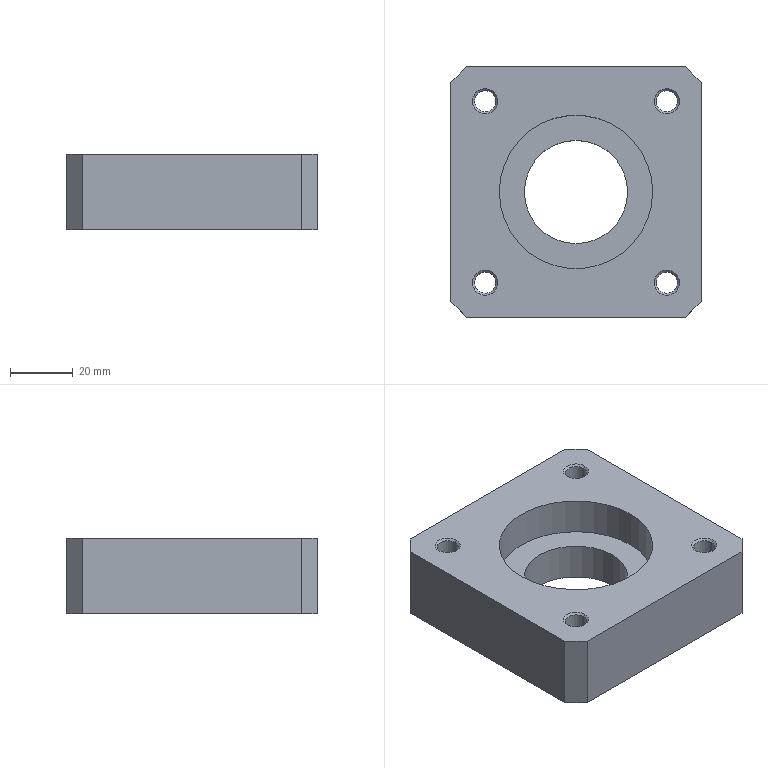Part | SolidWorks | features HoleWzd 2, Chamfer 1, Extrusion 1 | 1 solid | 31 faces | box 80 x 80 x 24 mm | volume 116003 mm3 | cylinder 12 | plane 11 | cone 8 | commonest cylinder face diameters 6.8 x8 33 x2 49 x2
STEP:
#1=CARTESIAN_POINT('',(-44.969,47.618,23.375));
#2=VERTEX_POINT('',#1);
#3=CARTESIAN_POINT('',(-38.169,47.618,23.375));
#4=VERTEX_POINT('',#3);
#5=CARTESIAN_POINT('',(-41.569,47.618,23.375));
#6=DIRECTION('',(0.,0.,1.));
#7=DIRECTION('',(1.,0.,0.));
#8=AXIS2_PLACEMENT_3D('',#5,#6,#7);
#9=CIRCLE('',#8,3.4);
#10=EDGE_CURVE('',#2,#4,#9,.T.);
#11=ORIENTED_EDGE('',*,*,#10,.F.);
#12=CARTESIAN_POINT('',(-45.594,47.618,24.));
#13=VERTEX_POINT('',#12);
#14=CARTESIAN_POINT('',(-45.594,47.618,24.));
#15=DIRECTION('',(-0.7071,0.,0.7071));
#16=VECTOR('',#15,1000.);
#17=LINE('',#14,#16);
#18=EDGE_CURVE('',#2,#13,#17,.T.);
#19=ORIENTED_EDGE('',*,*,#18,.T.);
#20=CARTESIAN_POINT('',(-37.544,47.618,24.));
#21=VERTEX_POINT('',#20);
#22=CARTESIAN_POINT('',(-41.569,47.618,24.));
#23=DIRECTION('',(0.,0.,1.));
#24=DIRECTION('',(1.,0.,0.));
#25=AXIS2_PLACEMENT_3D('',#22,#23,#24);
#26=CIRCLE('',#25,4.025);
#27=EDGE_CURVE('',#13,#21,#26,.T.);
#28=ORIENTED_EDGE('',*,*,#27,.T.);
#29=CARTESIAN_POINT('',(-37.544,47.618,24.));
#30=DIRECTION('',(0.7071,0.,0.7071));
#31=VECTOR('',#30,1000.);
#32=LINE('',#29,#31);
#33=EDGE_CURVE('',#4,#21,#32,.T.);
#34=ORIENTED_EDGE('',*,*,#33,.F.);
#35=EDGE_LOOP('',(#11,#19,#28,#34));
#36=FACE_OUTER_BOUND('',#35,.T.);
#37=CARTESIAN_POINT('',(-41.569,47.618,24.));
#38=DIRECTION('',(0.,0.,1.));
#39=DIRECTION('',(1.,0.,0.));
#40=AXIS2_PLACEMENT_3D('',#37,#38,#39);
#41=CONICAL_SURFACE('',#40,4.025,0.7854);
#42=ADVANCED_FACE('',(#36),#41,.F.);
#43=CARTESIAN_POINT('',(-44.969,47.618,0.));
#44=VERTEX_POINT('',#43);
#45=CARTESIAN_POINT('',(-38.169,47.618,0.));
#46=VERTEX_POINT('',#45);
#47=CARTESIAN_POINT('',(-41.569,47.618,0.));
#48=DIRECTION('',(0.,0.,1.));
#49=DIRECTION('',(1.,0.,0.));
#50=AXIS2_PLACEMENT_3D('',#47,#48,#49);
#51=CIRCLE('',#50,3.4);
#52=EDGE_CURVE('',#44,#46,#51,.T.);
#53=ORIENTED_EDGE('',*,*,#52,.F.);
#54=CARTESIAN_POINT('',(-44.969,47.618,24.));
#55=DIRECTION('',(0.,0.,1.));
#56=VECTOR('',#55,1000.);
#57=LINE('',#54,#56);
#58=EDGE_CURVE('',#44,#2,#57,.T.);
#59=ORIENTED_EDGE('',*,*,#58,.T.);
#60=ORIENTED_EDGE('',*,*,#10,.T.);
#61=CARTESIAN_POINT('',(-38.169,47.618,24.));
#62=DIRECTION('',(0.,0.,1.));
#63=VECTOR('',#62,1000.);
#64=LINE('',#61,#63);
#65=EDGE_CURVE('',#46,#4,#64,.T.);
#66=ORIENTED_EDGE('',*,*,#65,.F.);
#67=EDGE_LOOP('',(#53,#59,#60,#66));
#68=FACE_OUTER_BOUND('',#67,.T.);
#69=CARTESIAN_POINT('',(-41.569,47.618,24.));
#70=DIRECTION('',(0.,0.,1.));
#71=DIRECTION('',(1.,0.,0.));
#72=AXIS2_PLACEMENT_3D('',#69,#70,#71);
#73=CYLINDRICAL_SURFACE('',#72,3.4);
#74=ADVANCED_FACE('',(#68),#73,.F.);
#75=CARTESIAN_POINT('',(13.031,47.618,23.375));
#76=VERTEX_POINT('',#75);
#77=CARTESIAN_POINT('',(19.831,47.618,23.375));
#78=VERTEX_POINT('',#77);
#79=CARTESIAN_POINT('',(16.431,47.618,23.375));
#80=DIRECTION('',(0.,0.,1.));
#81=DIRECTION('',(1.,0.,0.));
#82=AXIS2_PLACEMENT_3D('',#79,#80,#81);
#83=CIRCLE('',#82,3.4);
#84=EDGE_CURVE('',#76,#78,#83,.T.);
#85=ORIENTED_EDGE('',*,*,#84,.F.);
#86=CARTESIAN_POINT('',(12.406,47.618,24.));
#87=VERTEX_POINT('',#86);
#88=CARTESIAN_POINT('',(12.406,47.618,24.));
#89=DIRECTION('',(-0.7071,0.,0.7071));
#90=VECTOR('',#89,1000.);
#91=LINE('',#88,#90);
#92=EDGE_CURVE('',#76,#87,#91,.T.);
#93=ORIENTED_EDGE('',*,*,#92,.T.);
#94=CARTESIAN_POINT('',(20.456,47.618,24.));
#95=VERTEX_POINT('',#94);
#96=CARTESIAN_POINT('',(16.431,47.618,24.));
#97=DIRECTION('',(0.,0.,1.));
#98=DIRECTION('',(1.,0.,0.));
#99=AXIS2_PLACEMENT_3D('',#96,#97,#98);
#100=CIRCLE('',#99,4.025);
#101=EDGE_CURVE('',#87,#95,#100,.T.);
#102=ORIENTED_EDGE('',*,*,#101,.T.);
#103=CARTESIAN_POINT('',(20.456,47.618,24.));
#104=DIRECTION('',(0.7071,0.,0.7071));
#105=VECTOR('',#104,1000.);
#106=LINE('',#103,#105);
#107=EDGE_CURVE('',#78,#95,#106,.T.);
#108=ORIENTED_EDGE('',*,*,#107,.F.);
#109=EDGE_LOOP('',(#85,#93,#102,#108));
#110=FACE_OUTER_BOUND('',#109,.T.);
#111=CARTESIAN_POINT('',(16.431,47.618,24.));
#112=DIRECTION('',(0.,0.,1.));
#113=DIRECTION('',(1.,0.,0.));
#114=AXIS2_PLACEMENT_3D('',#111,#112,#113);
#115=CONICAL_SURFACE('',#114,4.025,0.7854);
#116=ADVANCED_FACE('',(#110),#115,.F.);
#117=CARTESIAN_POINT('',(13.031,47.618,0.));
#118=VERTEX_POINT('',#117);
#119=CARTESIAN_POINT('',(19.831,47.618,0.));
#120=VERTEX_POINT('',#119);
#121=CARTESIAN_POINT('',(16.431,47.618,0.));
#122=DIRECTION('',(0.,0.,1.));
#123=DIRECTION('',(1.,0.,0.));
#124=AXIS2_PLACEMENT_3D('',#121,#122,#123);
#125=CIRCLE('',#124,3.4);
#126=EDGE_CURVE('',#118,#120,#125,.T.);
#127=ORIENTED_EDGE('',*,*,#126,.F.);
#128=CARTESIAN_POINT('',(13.031,47.618,24.));
#129=DIRECTION('',(0.,0.,1.));
#130=VECTOR('',#129,1000.);
#131=LINE('',#128,#130);
#132=EDGE_CURVE('',#118,#76,#131,.T.);
#133=ORIENTED_EDGE('',*,*,#132,.T.);
#134=ORIENTED_EDGE('',*,*,#84,.T.);
#135=CARTESIAN_POINT('',(19.831,47.618,24.));
#136=DIRECTION('',(0.,0.,1.));
#137=VECTOR('',#136,1000.);
#138=LINE('',#135,#137);
#139=EDGE_CURVE('',#120,#78,#138,.T.);
#140=ORIENTED_EDGE('',*,*,#139,.F.);
#141=EDGE_LOOP('',(#127,#133,#134,#140));
#142=FACE_OUTER_BOUND('',#141,.T.);
#143=CARTESIAN_POINT('',(16.431,47.618,24.));
#144=DIRECTION('',(0.,0.,1.));
#145=DIRECTION('',(1.,0.,0.));
#146=AXIS2_PLACEMENT_3D('',#143,#144,#145);
#147=CYLINDRICAL_SURFACE('',#146,3.4);
#148=ADVANCED_FACE('',(#142),#147,.F.);
#149=CARTESIAN_POINT('',(13.031,-10.382,23.375));
#150=VERTEX_POINT('',#149);
#151=CARTESIAN_POINT('',(19.831,-10.382,23.375));
#152=VERTEX_POINT('',#151);
#153=CARTESIAN_POINT('',(16.431,-10.382,23.375));
#154=DIRECTION('',(0.,0.,1.));
#155=DIRECTION('',(1.,0.,0.));
#156=AXIS2_PLACEMENT_3D('',#153,#154,#155);
#157=CIRCLE('',#156,3.4);
#158=EDGE_CURVE('',#150,#152,#157,.T.);
#159=ORIENTED_EDGE('',*,*,#158,.F.);
#160=CARTESIAN_POINT('',(12.406,-10.382,24.));
#161=VERTEX_POINT('',#160);
#162=CARTESIAN_POINT('',(12.406,-10.382,24.));
#163=DIRECTION('',(-0.7071,0.,0.7071));
#164=VECTOR('',#163,1000.);
#165=LINE('',#162,#164);
#166=EDGE_CURVE('',#150,#161,#165,.T.);
#167=ORIENTED_EDGE('',*,*,#166,.T.);
#168=CARTESIAN_POINT('',(20.456,-10.382,24.));
#169=VERTEX_POINT('',#168);
#170=CARTESIAN_POINT('',(16.431,-10.382,24.));
#171=DIRECTION('',(0.,0.,1.));
#172=DIRECTION('',(1.,0.,0.));
#173=AXIS2_PLACEMENT_3D('',#170,#171,#172);
#174=CIRCLE('',#173,4.025);
#175=EDGE_CURVE('',#161,#169,#174,.T.);
#176=ORIENTED_EDGE('',*,*,#175,.T.);
#177=CARTESIAN_POINT('',(20.456,-10.382,24.));
#178=DIRECTION('',(0.7071,0.,0.7071));
#179=VECTOR('',#178,1000.);
#180=LINE('',#177,#179);
#181=EDGE_CURVE('',#152,#169,#180,.T.);
#182=ORIENTED_EDGE('',*,*,#181,.F.);
#183=EDGE_LOOP('',(#159,#167,#176,#182));
#184=FACE_OUTER_BOUND('',#183,.T.);
#185=CARTESIAN_POINT('',(16.431,-10.382,24.));
#186=DIRECTION('',(0.,0.,1.));
#187=DIRECTION('',(1.,0.,0.));
#188=AXIS2_PLACEMENT_3D('',#185,#186,#187);
#189=CONICAL_SURFACE('',#188,4.025,0.7854);
#190=ADVANCED_FACE('',(#184),#189,.F.);
#191=CARTESIAN_POINT('',(13.031,-10.382,0.));
#192=VERTEX_POINT('',#191);
#193=CARTESIAN_POINT('',(19.831,-10.382,0.));
#194=VERTEX_POINT('',#193);
#195=CARTESIAN_POINT('',(16.431,-10.382,0.));
#196=DIRECTION('',(0.,0.,1.));
#197=DIRECTION('',(1.,0.,0.));
#198=AXIS2_PLACEMENT_3D('',#195,#196,#197);
#199=CIRCLE('',#198,3.4);
#200=EDGE_CURVE('',#192,#194,#199,.T.);
#201=ORIENTED_EDGE('',*,*,#200,.F.);
#202=CARTESIAN_POINT('',(13.031,-10.382,24.));
#203=DIRECTION('',(0.,0.,1.));
#204=VECTOR('',#203,1000.);
#205=LINE('',#202,#204);
#206=EDGE_CURVE('',#192,#150,#205,.T.);
#207=ORIENTED_EDGE('',*,*,#206,.T.);
#208=ORIENTED_EDGE('',*,*,#158,.T.);
#209=CARTESIAN_POINT('',(19.831,-10.382,24.));
#210=DIRECTION('',(0.,0.,1.));
#211=VECTOR('',#210,1000.);
#212=LINE('',#209,#211);
#213=EDGE_CURVE('',#194,#152,#212,.T.);
#214=ORIENTED_EDGE('',*,*,#213,.F.);
#215=EDGE_LOOP('',(#201,#207,#208,#214));
#216=FACE_OUTER_BOUND('',#215,.T.);
#217=CARTESIAN_POINT('',(16.431,-10.382,24.));
#218=DIRECTION('',(0.,0.,1.));
#219=DIRECTION('',(1.,0.,0.));
#220=AXIS2_PLACEMENT_3D('',#217,#218,#219);
#221=CYLINDRICAL_SURFACE('',#220,3.4);
#222=ADVANCED_FACE('',(#216),#221,.F.);
#223=CARTESIAN_POINT('',(-44.969,-10.382,23.375));
#224=VERTEX_POINT('',#223);
#225=CARTESIAN_POINT('',(-38.169,-10.382,23.375));
#226=VERTEX_POINT('',#225);
#227=CARTESIAN_POINT('',(-41.569,-10.382,23.375));
#228=DIRECTION('',(0.,0.,1.));
#229=DIRECTION('',(1.,0.,0.));
#230=AXIS2_PLACEMENT_3D('',#227,#228,#229);
#231=CIRCLE('',#230,3.4);
#232=EDGE_CURVE('',#224,#226,#231,.T.);
#233=ORIENTED_EDGE('',*,*,#232,.F.);
#234=CARTESIAN_POINT('',(-45.594,-10.382,24.));
#235=VERTEX_POINT('',#234);
#236=CARTESIAN_POINT('',(-45.594,-10.382,24.));
#237=DIRECTION('',(-0.7071,0.,0.7071));
#238=VECTOR('',#237,1000.);
#239=LINE('',#236,#238);
#240=EDGE_CURVE('',#224,#235,#239,.T.);
#241=ORIENTED_EDGE('',*,*,#240,.T.);
#242=CARTESIAN_POINT('',(-37.544,-10.382,24.));
#243=VERTEX_POINT('',#242);
#244=CARTESIAN_POINT('',(-41.569,-10.382,24.));
#245=DIRECTION('',(0.,0.,1.));
#246=DIRECTION('',(1.,0.,0.));
#247=AXIS2_PLACEMENT_3D('',#244,#245,#246);
#248=CIRCLE('',#247,4.025);
#249=EDGE_CURVE('',#235,#243,#248,.T.);
#250=ORIENTED_EDGE('',*,*,#249,.T.);
#251=CARTESIAN_POINT('',(-37.544,-10.382,24.));
#252=DIRECTION('',(0.7071,0.,0.7071));
#253=VECTOR('',#252,1000.);
#254=LINE('',#251,#253);
#255=EDGE_CURVE('',#226,#243,#254,.T.);
#256=ORIENTED_EDGE('',*,*,#255,.F.);
#257=EDGE_LOOP('',(#233,#241,#250,#256));
#258=FACE_OUTER_BOUND('',#257,.T.);
#259=CARTESIAN_POINT('',(-41.569,-10.382,24.));
#260=DIRECTION('',(0.,0.,1.));
#261=DIRECTION('',(1.,0.,0.));
#262=AXIS2_PLACEMENT_3D('',#259,#260,#261);
#263=CONICAL_SURFACE('',#262,4.025,0.7854);
#264=ADVANCED_FACE('',(#258),#263,.F.);
#265=CARTESIAN_POINT('',(-44.969,-10.382,0.));
#266=VERTEX_POINT('',#265);
#267=CARTESIAN_POINT('',(-38.169,-10.382,0.));
#268=VERTEX_POINT('',#267);
#269=CARTESIAN_POINT('',(-41.569,-10.382,0.));
#270=DIRECTION('',(0.,0.,1.));
#271=DIRECTION('',(1.,0.,0.));
#272=AXIS2_PLACEMENT_3D('',#269,#270,#271);
#273=CIRCLE('',#272,3.4);
#274=EDGE_CURVE('',#266,#268,#273,.T.);
#275=ORIENTED_EDGE('',*,*,#274,.F.);
#276=CARTESIAN_POINT('',(-44.969,-10.382,24.));
#277=DIRECTION('',(0.,0.,1.));
#278=VECTOR('',#277,1000.);
#279=LINE('',#276,#278);
#280=EDGE_CURVE('',#266,#224,#279,.T.);
#281=ORIENTED_EDGE('',*,*,#280,.T.);
#282=ORIENTED_EDGE('',*,*,#232,.T.);
#283=CARTESIAN_POINT('',(-38.169,-10.382,24.));
#284=DIRECTION('',(0.,0.,1.));
#285=VECTOR('',#284,1000.);
#286=LINE('',#283,#285);
#287=EDGE_CURVE('',#268,#226,#286,.T.);
#288=ORIENTED_EDGE('',*,*,#287,.F.);
#289=EDGE_LOOP('',(#275,#281,#282,#288));
#290=FACE_OUTER_BOUND('',#289,.T.);
#291=CARTESIAN_POINT('',(-41.569,-10.382,24.));
#292=DIRECTION('',(0.,0.,1.));
#293=DIRECTION('',(1.,0.,0.));
#294=AXIS2_PLACEMENT_3D('',#291,#292,#293);
#295=CYLINDRICAL_SURFACE('',#294,3.4);
#296=ADVANCED_FACE('',(#290),#295,.F.);
#297=CARTESIAN_POINT('',(-37.069,18.618,12.));
#298=VERTEX_POINT('',#297);
#299=CARTESIAN_POINT('',(11.931,18.618,12.));
#300=VERTEX_POINT('',#299);
#301=CARTESIAN_POINT('',(-12.569,18.618,12.));
#302=DIRECTION('',(0.,0.,1.));
#303=DIRECTION('',(1.,0.,0.));
#304=AXIS2_PLACEMENT_3D('',#301,#302,#303);
#305=CIRCLE('',#304,24.5);
#306=EDGE_CURVE('',#298,#300,#305,.T.);
#307=ORIENTED_EDGE('',*,*,#306,.F.);
#308=CARTESIAN_POINT('',(-37.069,18.618,24.));
#309=VERTEX_POINT('',#308);
#310=CARTESIAN_POINT('',(-37.069,18.618,24.));
#311=DIRECTION('',(0.,0.,1.));
#312=VECTOR('',#311,1000.);
#313=LINE('',#310,#312);
#314=EDGE_CURVE('',#298,#309,#313,.T.);
#315=ORIENTED_EDGE('',*,*,#314,.T.);
#316=CARTESIAN_POINT('',(11.931,18.618,24.));
#317=VERTEX_POINT('',#316);
#318=CARTESIAN_POINT('',(-12.569,18.618,24.));
#319=DIRECTION('',(0.,0.,1.));
#320=DIRECTION('',(1.,0.,0.));
#321=AXIS2_PLACEMENT_3D('',#318,#319,#320);
#322=CIRCLE('',#321,24.5);
#323=EDGE_CURVE('',#309,#317,#322,.T.);
#324=ORIENTED_EDGE('',*,*,#323,.T.);
#325=CARTESIAN_POINT('',(11.931,18.618,24.));
#326=DIRECTION('',(0.,0.,1.));
#327=VECTOR('',#326,1000.);
#328=LINE('',#325,#327);
#329=EDGE_CURVE('',#300,#317,#328,.T.);
#330=ORIENTED_EDGE('',*,*,#329,.F.);
#331=EDGE_LOOP('',(#307,#315,#324,#330));
#332=FACE_OUTER_BOUND('',#331,.T.);
#333=CARTESIAN_POINT('',(-12.569,18.618,24.));
#334=DIRECTION('',(0.,0.,1.));
#335=DIRECTION('',(1.,0.,0.));
#336=AXIS2_PLACEMENT_3D('',#333,#334,#335);
#337=CYLINDRICAL_SURFACE('',#336,24.5);
#338=ADVANCED_FACE('',(#332),#337,.F.);
#339=CARTESIAN_POINT('',(-29.069,18.618,0.));
#340=VERTEX_POINT('',#339);
#341=CARTESIAN_POINT('',(3.931,18.618,0.));
#342=VERTEX_POINT('',#341);
#343=CARTESIAN_POINT('',(-12.569,18.618,0.));
#344=DIRECTION('',(0.,0.,1.));
#345=DIRECTION('',(1.,0.,0.));
#346=AXIS2_PLACEMENT_3D('',#343,#344,#345);
#347=CIRCLE('',#346,16.5);
#348=EDGE_CURVE('',#340,#342,#347,.T.);
#349=ORIENTED_EDGE('',*,*,#348,.F.);
#350=CARTESIAN_POINT('',(-29.069,18.618,12.));
#351=VERTEX_POINT('',#350);
#352=CARTESIAN_POINT('',(-29.069,18.618,24.));
#353=DIRECTION('',(0.,0.,1.));
#354=VECTOR('',#353,1000.);
#355=LINE('',#352,#354);
#356=EDGE_CURVE('',#340,#351,#355,.T.);
#357=ORIENTED_EDGE('',*,*,#356,.T.);
#358=CARTESIAN_POINT('',(3.931,18.618,12.));
#359=VERTEX_POINT('',#358);
#360=CARTESIAN_POINT('',(-12.569,18.618,12.));
#361=DIRECTION('',(0.,0.,1.));
#362=DIRECTION('',(1.,0.,0.));
#363=AXIS2_PLACEMENT_3D('',#360,#361,#362);
#364=CIRCLE('',#363,16.5);
#365=EDGE_CURVE('',#351,#359,#364,.T.);
#366=ORIENTED_EDGE('',*,*,#365,.T.);
#367=CARTESIAN_POINT('',(3.931,18.618,24.));
#368=DIRECTION('',(0.,0.,1.));
#369=VECTOR('',#368,1000.);
#370=LINE('',#367,#369);
#371=EDGE_CURVE('',#342,#359,#370,.T.);
#372=ORIENTED_EDGE('',*,*,#371,.F.);
#373=EDGE_LOOP('',(#349,#357,#366,#372));
#374=FACE_OUTER_BOUND('',#373,.T.);
#375=CARTESIAN_POINT('',(-12.569,18.618,24.));
#376=DIRECTION('',(0.,0.,1.));
#377=DIRECTION('',(1.,0.,0.));
#378=AXIS2_PLACEMENT_3D('',#375,#376,#377);
#379=CYLINDRICAL_SURFACE('',#378,16.5);
#380=ADVANCED_FACE('',(#374),#379,.F.);
#381=CARTESIAN_POINT('',(-52.569,53.618,0.));
#382=VERTEX_POINT('',#381);
#383=CARTESIAN_POINT('',(-52.569,-16.382,0.));
#384=VERTEX_POINT('',#383);
#385=CARTESIAN_POINT('',(-52.569,58.618,0.));
#386=DIRECTION('',(0.,-1.,0.));
#387=VECTOR('',#386,1000.);
#388=LINE('',#385,#387);
#389=EDGE_CURVE('',#382,#384,#388,.T.);
#390=ORIENTED_EDGE('',*,*,#389,.T.);
#391=CARTESIAN_POINT('',(-52.569,-16.382,24.));
#392=VERTEX_POINT('',#391);
#393=CARTESIAN_POINT('',(-52.569,-16.382,24.));
#394=DIRECTION('',(0.,0.,1.));
#395=VECTOR('',#394,1000.);
#396=LINE('',#393,#395);
#397=EDGE_CURVE('',#384,#392,#396,.T.);
#398=ORIENTED_EDGE('',*,*,#397,.T.);
#399=CARTESIAN_POINT('',(-52.569,53.618,24.));
#400=VERTEX_POINT('',#399);
#401=CARTESIAN_POINT('',(-52.569,58.618,24.));
#402=DIRECTION('',(0.,-1.,0.));
#403=VECTOR('',#402,1000.);
#404=LINE('',#401,#403);
#405=EDGE_CURVE('',#400,#392,#404,.T.);
#406=ORIENTED_EDGE('',*,*,#405,.F.);
#407=CARTESIAN_POINT('',(-52.569,53.618,24.));
#408=DIRECTION('',(0.,0.,-1.));
#409=VECTOR('',#408,1000.);
#410=LINE('',#407,#409);
#411=EDGE_CURVE('',#400,#382,#410,.T.);
#412=ORIENTED_EDGE('',*,*,#411,.T.);
#413=EDGE_LOOP('',(#390,#398,#406,#412));
#414=FACE_OUTER_BOUND('',#413,.T.);
#415=CARTESIAN_POINT('',(-52.569,58.618,24.));
#416=DIRECTION('',(1.,0.,0.));
#417=DIRECTION('',(0.,1.,0.));
#418=AXIS2_PLACEMENT_3D('',#415,#416,#417);
#419=PLANE('',#418);
#420=ADVANCED_FACE('',(#414),#419,.F.);
#421=CARTESIAN_POINT('',(-47.569,-21.382,0.));
#422=VERTEX_POINT('',#421);
#423=CARTESIAN_POINT('',(22.431,-21.382,0.));
#424=VERTEX_POINT('',#423);
#425=CARTESIAN_POINT('',(-52.569,-21.382,0.));
#426=DIRECTION('',(1.,0.,0.));
#427=VECTOR('',#426,1000.);
#428=LINE('',#425,#427);
#429=EDGE_CURVE('',#422,#424,#428,.T.);
#430=ORIENTED_EDGE('',*,*,#429,.T.);
#431=CARTESIAN_POINT('',(22.431,-21.382,24.));
#432=VERTEX_POINT('',#431);
#433=CARTESIAN_POINT('',(22.431,-21.382,24.));
#434=DIRECTION('',(0.,0.,1.));
#435=VECTOR('',#434,1000.);
#436=LINE('',#433,#435);
#437=EDGE_CURVE('',#424,#432,#436,.T.);
#438=ORIENTED_EDGE('',*,*,#437,.T.);
#439=CARTESIAN_POINT('',(-47.569,-21.382,24.));
#440=VERTEX_POINT('',#439);
#441=CARTESIAN_POINT('',(-52.569,-21.382,24.));
#442=DIRECTION('',(1.,0.,0.));
#443=VECTOR('',#442,1000.);
#444=LINE('',#441,#443);
#445=EDGE_CURVE('',#440,#432,#444,.T.);
#446=ORIENTED_EDGE('',*,*,#445,.F.);
#447=CARTESIAN_POINT('',(-47.569,-21.382,24.));
#448=DIRECTION('',(0.,0.,-1.));
#449=VECTOR('',#448,1000.);
#450=LINE('',#447,#449);
#451=EDGE_CURVE('',#440,#422,#450,.T.);
#452=ORIENTED_EDGE('',*,*,#451,.T.);
#453=EDGE_LOOP('',(#430,#438,#446,#452));
#454=FACE_OUTER_BOUND('',#453,.T.);
#455=CARTESIAN_POINT('',(-52.569,-21.382,24.));
#456=DIRECTION('',(0.,1.,0.));
#457=DIRECTION('',(0.,0.,1.));
#458=AXIS2_PLACEMENT_3D('',#455,#456,#457);
#459=PLANE('',#458);
#460=ADVANCED_FACE('',(#454),#459,.F.);
#461=CARTESIAN_POINT('',(27.431,-16.382,0.));
#462=VERTEX_POINT('',#461);
#463=CARTESIAN_POINT('',(27.431,53.618,0.));
#464=VERTEX_POINT('',#463);
#465=CARTESIAN_POINT('',(27.431,58.618,0.));
#466=DIRECTION('',(0.,1.,0.));
#467=VECTOR('',#466,1000.);
#468=LINE('',#465,#467);
#469=EDGE_CURVE('',#462,#464,#468,.T.);
#470=ORIENTED_EDGE('',*,*,#469,.T.);
#471=CARTESIAN_POINT('',(27.431,53.618,24.));
#472=VERTEX_POINT('',#471);
#473=CARTESIAN_POINT('',(27.431,53.618,24.));
#474=DIRECTION('',(0.,0.,1.));
#475=VECTOR('',#474,1000.);
#476=LINE('',#473,#475);
#477=EDGE_CURVE('',#464,#472,#476,.T.);
#478=ORIENTED_EDGE('',*,*,#477,.T.);
#479=CARTESIAN_POINT('',(27.431,-16.382,24.));
#480=VERTEX_POINT('',#479);
#481=CARTESIAN_POINT('',(27.431,58.618,24.));
#482=DIRECTION('',(0.,1.,0.));
#483=VECTOR('',#482,1000.);
#484=LINE('',#481,#483);
#485=EDGE_CURVE('',#480,#472,#484,.T.);
#486=ORIENTED_EDGE('',*,*,#485,.F.);
#487=CARTESIAN_POINT('',(27.431,-16.382,24.));
#488=DIRECTION('',(0.,0.,-1.));
#489=VECTOR('',#488,1000.);
#490=LINE('',#487,#489);
#491=EDGE_CURVE('',#480,#462,#490,.T.);
#492=ORIENTED_EDGE('',*,*,#491,.T.);
#493=EDGE_LOOP('',(#470,#478,#486,#492));
#494=FACE_OUTER_BOUND('',#493,.T.);
#495=CARTESIAN_POINT('',(27.431,58.618,24.));
#496=DIRECTION('',(-1.,0.,0.));
#497=DIRECTION('',(0.,-1.,0.));
#498=AXIS2_PLACEMENT_3D('',#495,#496,#497);
#499=PLANE('',#498);
#500=ADVANCED_FACE('',(#494),#499,.F.);
#501=CARTESIAN_POINT('',(22.431,58.618,24.));
#502=VERTEX_POINT('',#501);
#503=CARTESIAN_POINT('',(-47.569,58.618,24.));
#504=VERTEX_POINT('',#503);
#505=CARTESIAN_POINT('',(-52.569,58.618,24.));
#506=DIRECTION('',(-1.,0.,0.));
#507=VECTOR('',#506,1000.);
#508=LINE('',#505,#507);
#509=EDGE_CURVE('',#502,#504,#508,.T.);
#510=ORIENTED_EDGE('',*,*,#509,.F.);
#511=CARTESIAN_POINT('',(22.431,58.618,0.));
#512=VERTEX_POINT('',#511);
#513=CARTESIAN_POINT('',(22.431,58.618,24.));
#514=DIRECTION('',(0.,0.,-1.));
#515=VECTOR('',#514,1000.);
#516=LINE('',#513,#515);
#517=EDGE_CURVE('',#502,#512,#516,.T.);
#518=ORIENTED_EDGE('',*,*,#517,.T.);
#519=CARTESIAN_POINT('',(-47.569,58.618,0.));
#520=VERTEX_POINT('',#519);
#521=CARTESIAN_POINT('',(-52.569,58.618,0.));
#522=DIRECTION('',(-1.,0.,0.));
#523=VECTOR('',#522,1000.);
#524=LINE('',#521,#523);
#525=EDGE_CURVE('',#512,#520,#524,.T.);
#526=ORIENTED_EDGE('',*,*,#525,.T.);
#527=CARTESIAN_POINT('',(-47.569,58.618,24.));
#528=DIRECTION('',(0.,0.,1.));
#529=VECTOR('',#528,1000.);
#530=LINE('',#527,#529);
#531=EDGE_CURVE('',#520,#504,#530,.T.);
#532=ORIENTED_EDGE('',*,*,#531,.T.);
#533=EDGE_LOOP('',(#510,#518,#526,#532));
#534=FACE_OUTER_BOUND('',#533,.T.);
#535=CARTESIAN_POINT('',(-52.569,58.618,24.));
#536=DIRECTION('',(0.,-1.,0.));
#537=DIRECTION('',(0.,0.,-1.));
#538=AXIS2_PLACEMENT_3D('',#535,#536,#537);
#539=PLANE('',#538);
#540=ADVANCED_FACE('',(#534),#539,.F.);
#541=CARTESIAN_POINT('',(-41.569,47.618,24.));
#542=DIRECTION('',(0.,0.,1.));
#543=DIRECTION('',(1.,0.,0.));
#544=AXIS2_PLACEMENT_3D('',#541,#542,#543);
#545=CIRCLE('',#544,4.025);
#546=EDGE_CURVE('',#21,#13,#545,.T.);
#547=ORIENTED_EDGE('',*,*,#546,.F.);
#548=ORIENTED_EDGE('',*,*,#27,.F.);
#549=EDGE_LOOP('',(#547,#548));
#550=FACE_BOUND('',#549,.T.);
#551=CARTESIAN_POINT('',(16.431,47.618,24.));
#552=DIRECTION('',(0.,0.,1.));
#553=DIRECTION('',(1.,0.,0.));
#554=AXIS2_PLACEMENT_3D('',#551,#552,#553);
#555=CIRCLE('',#554,4.025);
#556=EDGE_CURVE('',#95,#87,#555,.T.);
#557=ORIENTED_EDGE('',*,*,#556,.F.);
#558=ORIENTED_EDGE('',*,*,#101,.F.);
#559=EDGE_LOOP('',(#557,#558));
#560=FACE_BOUND('',#559,.T.);
#561=CARTESIAN_POINT('',(16.431,-10.382,24.));
#562=DIRECTION('',(0.,0.,1.));
#563=DIRECTION('',(1.,0.,0.));
#564=AXIS2_PLACEMENT_3D('',#561,#562,#563);
#565=CIRCLE('',#564,4.025);
#566=EDGE_CURVE('',#169,#161,#565,.T.);
#567=ORIENTED_EDGE('',*,*,#566,.F.);
#568=ORIENTED_EDGE('',*,*,#175,.F.);
#569=EDGE_LOOP('',(#567,#568));
#570=FACE_BOUND('',#569,.T.);
#571=CARTESIAN_POINT('',(-41.569,-10.382,24.));
#572=DIRECTION('',(0.,0.,1.));
#573=DIRECTION('',(1.,0.,0.));
#574=AXIS2_PLACEMENT_3D('',#571,#572,#573);
#575=CIRCLE('',#574,4.025);
#576=EDGE_CURVE('',#243,#235,#575,.T.);
#577=ORIENTED_EDGE('',*,*,#576,.F.);
#578=ORIENTED_EDGE('',*,*,#249,.F.);
#579=EDGE_LOOP('',(#577,#578));
#580=FACE_BOUND('',#579,.T.);
#581=CARTESIAN_POINT('',(-12.569,18.618,24.));
#582=DIRECTION('',(0.,0.,1.));
#583=DIRECTION('',(1.,0.,0.));
#584=AXIS2_PLACEMENT_3D('',#581,#582,#583);
#585=CIRCLE('',#584,24.5);
#586=EDGE_CURVE('',#317,#309,#585,.T.);
#587=ORIENTED_EDGE('',*,*,#586,.F.);
#588=ORIENTED_EDGE('',*,*,#323,.F.);
#589=EDGE_LOOP('',(#587,#588));
#590=FACE_BOUND('',#589,.T.);
#591=ORIENTED_EDGE('',*,*,#485,.T.);
#592=CARTESIAN_POINT('',(40.525,40.525,24.));
#593=DIRECTION('',(-0.7071,0.7071,0.));
#594=VECTOR('',#593,1000.);
#595=LINE('',#592,#594);
#596=EDGE_CURVE('',#472,#502,#595,.T.);
#597=ORIENTED_EDGE('',*,*,#596,.T.);
#598=ORIENTED_EDGE('',*,*,#509,.T.);
#599=CARTESIAN_POINT('',(-53.094,53.094,24.));
#600=DIRECTION('',(-0.7071,-0.7071,0.));
#601=VECTOR('',#600,1000.);
#602=LINE('',#599,#601);
#603=EDGE_CURVE('',#504,#400,#602,.T.);
#604=ORIENTED_EDGE('',*,*,#603,.T.);
#605=ORIENTED_EDGE('',*,*,#405,.T.);
#606=CARTESIAN_POINT('',(-34.475,-34.475,24.));
#607=DIRECTION('',(0.7071,-0.7071,0.));
#608=VECTOR('',#607,1000.);
#609=LINE('',#606,#608);
#610=EDGE_CURVE('',#392,#440,#609,.T.);
#611=ORIENTED_EDGE('',*,*,#610,.T.);
#612=ORIENTED_EDGE('',*,*,#445,.T.);
#613=CARTESIAN_POINT('',(21.906,-21.906,24.));
#614=DIRECTION('',(0.7071,0.7071,0.));
#615=VECTOR('',#614,1000.);
#616=LINE('',#613,#615);
#617=EDGE_CURVE('',#432,#480,#616,.T.);
#618=ORIENTED_EDGE('',*,*,#617,.T.);
#619=EDGE_LOOP('',(#591,#597,#598,#604,#605,#611,#612,#618));
#620=FACE_OUTER_BOUND('',#619,.T.);
#621=CARTESIAN_POINT('',(0.,0.,24.));
#622=DIRECTION('',(0.,0.,1.));
#623=DIRECTION('',(1.,0.,0.));
#624=AXIS2_PLACEMENT_3D('',#621,#622,#623);
#625=PLANE('',#624);
#626=ADVANCED_FACE('',(#550,#560,#570,#580,#590,#620),#625,.T.);
#627=CARTESIAN_POINT('',(-41.569,47.618,0.));
#628=DIRECTION('',(0.,0.,1.));
#629=DIRECTION('',(1.,0.,0.));
#630=AXIS2_PLACEMENT_3D('',#627,#628,#629);
#631=CIRCLE('',#630,3.4);
#632=EDGE_CURVE('',#46,#44,#631,.T.);
#633=ORIENTED_EDGE('',*,*,#632,.T.);
#634=ORIENTED_EDGE('',*,*,#52,.T.);
#635=EDGE_LOOP('',(#633,#634));
#636=FACE_BOUND('',#635,.T.);
#637=CARTESIAN_POINT('',(16.431,47.618,0.));
#638=DIRECTION('',(0.,0.,1.));
#639=DIRECTION('',(1.,0.,0.));
#640=AXIS2_PLACEMENT_3D('',#637,#638,#639);
#641=CIRCLE('',#640,3.4);
#642=EDGE_CURVE('',#120,#118,#641,.T.);
#643=ORIENTED_EDGE('',*,*,#642,.T.);
#644=ORIENTED_EDGE('',*,*,#126,.T.);
#645=EDGE_LOOP('',(#643,#644));
#646=FACE_BOUND('',#645,.T.);
#647=CARTESIAN_POINT('',(16.431,-10.382,0.));
#648=DIRECTION('',(0.,0.,1.));
#649=DIRECTION('',(1.,0.,0.));
#650=AXIS2_PLACEMENT_3D('',#647,#648,#649);
#651=CIRCLE('',#650,3.4);
#652=EDGE_CURVE('',#194,#192,#651,.T.);
#653=ORIENTED_EDGE('',*,*,#652,.T.);
#654=ORIENTED_EDGE('',*,*,#200,.T.);
#655=EDGE_LOOP('',(#653,#654));
#656=FACE_BOUND('',#655,.T.);
#657=CARTESIAN_POINT('',(-41.569,-10.382,0.));
#658=DIRECTION('',(0.,0.,1.));
#659=DIRECTION('',(1.,0.,0.));
#660=AXIS2_PLACEMENT_3D('',#657,#658,#659);
#661=CIRCLE('',#660,3.4);
#662=EDGE_CURVE('',#268,#266,#661,.T.);
#663=ORIENTED_EDGE('',*,*,#662,.T.);
#664=ORIENTED_EDGE('',*,*,#274,.T.);
#665=EDGE_LOOP('',(#663,#664));
#666=FACE_BOUND('',#665,.T.);
#667=CARTESIAN_POINT('',(-12.569,18.618,0.));
#668=DIRECTION('',(0.,0.,1.));
#669=DIRECTION('',(1.,0.,0.));
#670=AXIS2_PLACEMENT_3D('',#667,#668,#669);
#671=CIRCLE('',#670,16.5);
#672=EDGE_CURVE('',#342,#340,#671,.T.);
#673=ORIENTED_EDGE('',*,*,#672,.T.);
#674=ORIENTED_EDGE('',*,*,#348,.T.);
#675=EDGE_LOOP('',(#673,#674));
#676=FACE_BOUND('',#675,.T.);
#677=ORIENTED_EDGE('',*,*,#525,.F.);
#678=CARTESIAN_POINT('',(22.431,58.618,0.));
#679=DIRECTION('',(0.7071,-0.7071,0.));
#680=VECTOR('',#679,1000.);
#681=LINE('',#678,#680);
#682=EDGE_CURVE('',#512,#464,#681,.T.);
#683=ORIENTED_EDGE('',*,*,#682,.T.);
#684=ORIENTED_EDGE('',*,*,#469,.F.);
#685=CARTESIAN_POINT('',(27.431,-16.382,0.));
#686=DIRECTION('',(-0.7071,-0.7071,0.));
#687=VECTOR('',#686,1000.);
#688=LINE('',#685,#687);
#689=EDGE_CURVE('',#462,#424,#688,.T.);
#690=ORIENTED_EDGE('',*,*,#689,.T.);
#691=ORIENTED_EDGE('',*,*,#429,.F.);
#692=CARTESIAN_POINT('',(-47.569,-21.382,0.));
#693=DIRECTION('',(-0.7071,0.7071,0.));
#694=VECTOR('',#693,1000.);
#695=LINE('',#692,#694);
#696=EDGE_CURVE('',#422,#384,#695,.T.);
#697=ORIENTED_EDGE('',*,*,#696,.T.);
#698=ORIENTED_EDGE('',*,*,#389,.F.);
#699=CARTESIAN_POINT('',(-52.569,53.618,0.));
#700=DIRECTION('',(0.7071,0.7071,0.));
#701=VECTOR('',#700,1000.);
#702=LINE('',#699,#701);
#703=EDGE_CURVE('',#382,#520,#702,.T.);
#704=ORIENTED_EDGE('',*,*,#703,.T.);
#705=EDGE_LOOP('',(#677,#683,#684,#690,#691,#697,#698,#704));
#706=FACE_OUTER_BOUND('',#705,.T.);
#707=CARTESIAN_POINT('',(0.,0.,0.));
#708=DIRECTION('',(0.,0.,1.));
#709=DIRECTION('',(1.,0.,0.));
#710=AXIS2_PLACEMENT_3D('',#707,#708,#709);
#711=PLANE('',#710);
#712=ADVANCED_FACE('',(#636,#646,#656,#666,#676,#706),#711,.F.);
#713=ORIENTED_EDGE('',*,*,#356,.F.);
#714=ORIENTED_EDGE('',*,*,#672,.F.);
#715=ORIENTED_EDGE('',*,*,#371,.T.);
#716=CARTESIAN_POINT('',(-12.569,18.618,12.));
#717=DIRECTION('',(0.,0.,1.));
#718=DIRECTION('',(1.,0.,0.));
#719=AXIS2_PLACEMENT_3D('',#716,#717,#718);
#720=CIRCLE('',#719,16.5);
#721=EDGE_CURVE('',#359,#351,#720,.T.);
#722=ORIENTED_EDGE('',*,*,#721,.T.);
#723=EDGE_LOOP('',(#713,#714,#715,#722));
#724=FACE_OUTER_BOUND('',#723,.T.);
#725=CARTESIAN_POINT('',(-12.569,18.618,24.));
#726=DIRECTION('',(0.,0.,1.));
#727=DIRECTION('',(1.,0.,0.));
#728=AXIS2_PLACEMENT_3D('',#725,#726,#727);
#729=CYLINDRICAL_SURFACE('',#728,16.5);
#730=ADVANCED_FACE('',(#724),#729,.F.);
#731=ORIENTED_EDGE('',*,*,#721,.F.);
#732=ORIENTED_EDGE('',*,*,#365,.F.);
#733=EDGE_LOOP('',(#731,#732));
#734=FACE_BOUND('',#733,.T.);
#735=CARTESIAN_POINT('',(-12.569,18.618,12.));
#736=DIRECTION('',(0.,0.,1.));
#737=DIRECTION('',(1.,0.,0.));
#738=AXIS2_PLACEMENT_3D('',#735,#736,#737);
#739=CIRCLE('',#738,24.5);
#740=EDGE_CURVE('',#300,#298,#739,.T.);
#741=ORIENTED_EDGE('',*,*,#740,.T.);
#742=ORIENTED_EDGE('',*,*,#306,.T.);
#743=EDGE_LOOP('',(#741,#742));
#744=FACE_OUTER_BOUND('',#743,.T.);
#745=CARTESIAN_POINT('',(3.931,18.618,12.));
#746=DIRECTION('',(0.,0.,-1.));
#747=DIRECTION('',(-1.,0.,0.));
#748=AXIS2_PLACEMENT_3D('',#745,#746,#747);
#749=PLANE('',#748);
#750=ADVANCED_FACE('',(#734,#744),#749,.F.);
#751=ORIENTED_EDGE('',*,*,#314,.F.);
#752=ORIENTED_EDGE('',*,*,#740,.F.);
#753=ORIENTED_EDGE('',*,*,#329,.T.);
#754=ORIENTED_EDGE('',*,*,#586,.T.);
#755=EDGE_LOOP('',(#751,#752,#753,#754));
#756=FACE_OUTER_BOUND('',#755,.T.);
#757=CARTESIAN_POINT('',(-12.569,18.618,24.));
#758=DIRECTION('',(0.,0.,1.));
#759=DIRECTION('',(1.,0.,0.));
#760=AXIS2_PLACEMENT_3D('',#757,#758,#759);
#761=CYLINDRICAL_SURFACE('',#760,24.5);
#762=ADVANCED_FACE('',(#756),#761,.F.);
#763=ORIENTED_EDGE('',*,*,#280,.F.);
#764=ORIENTED_EDGE('',*,*,#662,.F.);
#765=ORIENTED_EDGE('',*,*,#287,.T.);
#766=CARTESIAN_POINT('',(-41.569,-10.382,23.375));
#767=DIRECTION('',(0.,0.,1.));
#768=DIRECTION('',(1.,0.,0.));
#769=AXIS2_PLACEMENT_3D('',#766,#767,#768);
#770=CIRCLE('',#769,3.4);
#771=EDGE_CURVE('',#226,#224,#770,.T.);
#772=ORIENTED_EDGE('',*,*,#771,.T.);
#773=EDGE_LOOP('',(#763,#764,#765,#772));
#774=FACE_OUTER_BOUND('',#773,.T.);
#775=CARTESIAN_POINT('',(-41.569,-10.382,24.));
#776=DIRECTION('',(0.,0.,1.));
#777=DIRECTION('',(1.,0.,0.));
#778=AXIS2_PLACEMENT_3D('',#775,#776,#777);
#779=CYLINDRICAL_SURFACE('',#778,3.4);
#780=ADVANCED_FACE('',(#774),#779,.F.);
#781=ORIENTED_EDGE('',*,*,#240,.F.);
#782=ORIENTED_EDGE('',*,*,#771,.F.);
#783=ORIENTED_EDGE('',*,*,#255,.T.);
#784=ORIENTED_EDGE('',*,*,#576,.T.);
#785=EDGE_LOOP('',(#781,#782,#783,#784));
#786=FACE_OUTER_BOUND('',#785,.T.);
#787=CARTESIAN_POINT('',(-41.569,-10.382,24.));
#788=DIRECTION('',(0.,0.,1.));
#789=DIRECTION('',(1.,0.,0.));
#790=AXIS2_PLACEMENT_3D('',#787,#788,#789);
#791=CONICAL_SURFACE('',#790,4.025,0.7854);
#792=ADVANCED_FACE('',(#786),#791,.F.);
#793=ORIENTED_EDGE('',*,*,#206,.F.);
#794=ORIENTED_EDGE('',*,*,#652,.F.);
#795=ORIENTED_EDGE('',*,*,#213,.T.);
#796=CARTESIAN_POINT('',(16.431,-10.382,23.375));
#797=DIRECTION('',(0.,0.,1.));
#798=DIRECTION('',(1.,0.,0.));
#799=AXIS2_PLACEMENT_3D('',#796,#797,#798);
#800=CIRCLE('',#799,3.4);
#801=EDGE_CURVE('',#152,#150,#800,.T.);
#802=ORIENTED_EDGE('',*,*,#801,.T.);
#803=EDGE_LOOP('',(#793,#794,#795,#802));
#804=FACE_OUTER_BOUND('',#803,.T.);
#805=CARTESIAN_POINT('',(16.431,-10.382,24.));
#806=DIRECTION('',(0.,0.,1.));
#807=DIRECTION('',(1.,0.,0.));
#808=AXIS2_PLACEMENT_3D('',#805,#806,#807);
#809=CYLINDRICAL_SURFACE('',#808,3.4);
#810=ADVANCED_FACE('',(#804),#809,.F.);
#811=ORIENTED_EDGE('',*,*,#166,.F.);
#812=ORIENTED_EDGE('',*,*,#801,.F.);
#813=ORIENTED_EDGE('',*,*,#181,.T.);
#814=ORIENTED_EDGE('',*,*,#566,.T.);
#815=EDGE_LOOP('',(#811,#812,#813,#814));
#816=FACE_OUTER_BOUND('',#815,.T.);
#817=CARTESIAN_POINT('',(16.431,-10.382,24.));
#818=DIRECTION('',(0.,0.,1.));
#819=DIRECTION('',(1.,0.,0.));
#820=AXIS2_PLACEMENT_3D('',#817,#818,#819);
#821=CONICAL_SURFACE('',#820,4.025,0.7854);
#822=ADVANCED_FACE('',(#816),#821,.F.);
#823=ORIENTED_EDGE('',*,*,#132,.F.);
#824=ORIENTED_EDGE('',*,*,#642,.F.);
#825=ORIENTED_EDGE('',*,*,#139,.T.);
#826=CARTESIAN_POINT('',(16.431,47.618,23.375));
#827=DIRECTION('',(0.,0.,1.));
#828=DIRECTION('',(1.,0.,0.));
#829=AXIS2_PLACEMENT_3D('',#826,#827,#828);
#830=CIRCLE('',#829,3.4);
#831=EDGE_CURVE('',#78,#76,#830,.T.);
#832=ORIENTED_EDGE('',*,*,#831,.T.);
#833=EDGE_LOOP('',(#823,#824,#825,#832));
#834=FACE_OUTER_BOUND('',#833,.T.);
#835=CARTESIAN_POINT('',(16.431,47.618,24.));
#836=DIRECTION('',(0.,0.,1.));
#837=DIRECTION('',(1.,0.,0.));
#838=AXIS2_PLACEMENT_3D('',#835,#836,#837);
#839=CYLINDRICAL_SURFACE('',#838,3.4);
#840=ADVANCED_FACE('',(#834),#839,.F.);
#841=ORIENTED_EDGE('',*,*,#92,.F.);
#842=ORIENTED_EDGE('',*,*,#831,.F.);
#843=ORIENTED_EDGE('',*,*,#107,.T.);
#844=ORIENTED_EDGE('',*,*,#556,.T.);
#845=EDGE_LOOP('',(#841,#842,#843,#844));
#846=FACE_OUTER_BOUND('',#845,.T.);
#847=CARTESIAN_POINT('',(16.431,47.618,24.));
#848=DIRECTION('',(0.,0.,1.));
#849=DIRECTION('',(1.,0.,0.));
#850=AXIS2_PLACEMENT_3D('',#847,#848,#849);
#851=CONICAL_SURFACE('',#850,4.025,0.7854);
#852=ADVANCED_FACE('',(#846),#851,.F.);
#853=ORIENTED_EDGE('',*,*,#58,.F.);
#854=ORIENTED_EDGE('',*,*,#632,.F.);
#855=ORIENTED_EDGE('',*,*,#65,.T.);
#856=CARTESIAN_POINT('',(-41.569,47.618,23.375));
#857=DIRECTION('',(0.,0.,1.));
#858=DIRECTION('',(1.,0.,0.));
#859=AXIS2_PLACEMENT_3D('',#856,#857,#858);
#860=CIRCLE('',#859,3.4);
#861=EDGE_CURVE('',#4,#2,#860,.T.);
#862=ORIENTED_EDGE('',*,*,#861,.T.);
#863=EDGE_LOOP('',(#853,#854,#855,#862));
#864=FACE_OUTER_BOUND('',#863,.T.);
#865=CARTESIAN_POINT('',(-41.569,47.618,24.));
#866=DIRECTION('',(0.,0.,1.));
#867=DIRECTION('',(1.,0.,0.));
#868=AXIS2_PLACEMENT_3D('',#865,#866,#867);
#869=CYLINDRICAL_SURFACE('',#868,3.4);
#870=ADVANCED_FACE('',(#864),#869,.F.);
#871=ORIENTED_EDGE('',*,*,#18,.F.);
#872=ORIENTED_EDGE('',*,*,#861,.F.);
#873=ORIENTED_EDGE('',*,*,#33,.T.);
#874=ORIENTED_EDGE('',*,*,#546,.T.);
#875=EDGE_LOOP('',(#871,#872,#873,#874));
#876=FACE_OUTER_BOUND('',#875,.T.);
#877=CARTESIAN_POINT('',(-41.569,47.618,24.));
#878=DIRECTION('',(0.,0.,1.));
#879=DIRECTION('',(1.,0.,0.));
#880=AXIS2_PLACEMENT_3D('',#877,#878,#879);
#881=CONICAL_SURFACE('',#880,4.025,0.7854);
#882=ADVANCED_FACE('',(#876),#881,.F.);
#883=ORIENTED_EDGE('',*,*,#596,.F.);
#884=ORIENTED_EDGE('',*,*,#477,.F.);
#885=ORIENTED_EDGE('',*,*,#682,.F.);
#886=ORIENTED_EDGE('',*,*,#517,.F.);
#887=EDGE_LOOP('',(#883,#884,#885,#886));
#888=FACE_OUTER_BOUND('',#887,.T.);
#889=CARTESIAN_POINT('',(22.431,58.618,24.));
#890=DIRECTION('',(-0.7071,-0.7071,0.));
#891=DIRECTION('',(0.,0.,-1.));
#892=AXIS2_PLACEMENT_3D('',#889,#890,#891);
#893=PLANE('',#892);
#894=ADVANCED_FACE('',(#888),#893,.F.);
#895=ORIENTED_EDGE('',*,*,#617,.F.);
#896=ORIENTED_EDGE('',*,*,#437,.F.);
#897=ORIENTED_EDGE('',*,*,#689,.F.);
#898=ORIENTED_EDGE('',*,*,#491,.F.);
#899=EDGE_LOOP('',(#895,#896,#897,#898));
#900=FACE_OUTER_BOUND('',#899,.T.);
#901=CARTESIAN_POINT('',(27.431,-16.382,24.));
#902=DIRECTION('',(-0.7071,0.7071,0.));
#903=DIRECTION('',(0.,0.,-1.));
#904=AXIS2_PLACEMENT_3D('',#901,#902,#903);
#905=PLANE('',#904);
#906=ADVANCED_FACE('',(#900),#905,.F.);
#907=ORIENTED_EDGE('',*,*,#610,.F.);
#908=ORIENTED_EDGE('',*,*,#397,.F.);
#909=ORIENTED_EDGE('',*,*,#696,.F.);
#910=ORIENTED_EDGE('',*,*,#451,.F.);
#911=EDGE_LOOP('',(#907,#908,#909,#910));
#912=FACE_OUTER_BOUND('',#911,.T.);
#913=CARTESIAN_POINT('',(-47.569,-21.382,24.));
#914=DIRECTION('',(0.7071,0.7071,0.));
#915=DIRECTION('',(0.,0.,-1.));
#916=AXIS2_PLACEMENT_3D('',#913,#914,#915);
#917=PLANE('',#916);
#918=ADVANCED_FACE('',(#912),#917,.F.);
#919=ORIENTED_EDGE('',*,*,#603,.F.);
#920=ORIENTED_EDGE('',*,*,#531,.F.);
#921=ORIENTED_EDGE('',*,*,#703,.F.);
#922=ORIENTED_EDGE('',*,*,#411,.F.);
#923=EDGE_LOOP('',(#919,#920,#921,#922));
#924=FACE_OUTER_BOUND('',#923,.T.);
#925=CARTESIAN_POINT('',(-52.569,53.618,24.));
#926=DIRECTION('',(0.7071,-0.7071,0.));
#927=DIRECTION('',(0.,0.,-1.));
#928=AXIS2_PLACEMENT_3D('',#925,#926,#927);
#929=PLANE('',#928);
#930=ADVANCED_FACE('',(#924),#929,.F.);
#931=CLOSED_SHELL('',(#42,#74,#116,#148,#190,#222,#264,#296,#338,#380,#420,#460,#500,#540,#626,#712,#730,#750,#762,#780,#792,#810,#822,#840,#852,#870,#882,#894,#906,#918,#930));
#932=MANIFOLD_SOLID_BREP('',#931);
#933=CARTESIAN_POINT('',(0.,0.,0.));
#934=DIRECTION('',(0.,0.,1.));
#935=DIRECTION('',(1.,0.,0.));
#936=AXIS2_PLACEMENT_3D('',#933,#934,#935);
#937=(LENGTH_UNIT()NAMED_UNIT(*)SI_UNIT(.MILLI.,.METRE.));
#938=UNCERTAINTY_MEASURE_WITH_UNIT(LENGTH_MEASURE(0.00001),#937,'','');
#939=(NAMED_UNIT(*)PLANE_ANGLE_UNIT()SI_UNIT($,.RADIAN.));
#940=(NAMED_UNIT(*)SI_UNIT($,.STERADIAN.)SOLID_ANGLE_UNIT());
#941=(GEOMETRIC_REPRESENTATION_CONTEXT(3)GLOBAL_UNCERTAINTY_ASSIGNED_CONTEXT((#938))GLOBAL_UNIT_ASSIGNED_CONTEXT((#937,#939,#940))REPRESENTATION_CONTEXT('',''));
#942=ADVANCED_BREP_SHAPE_REPRESENTATION('',(#932,#936),#941);